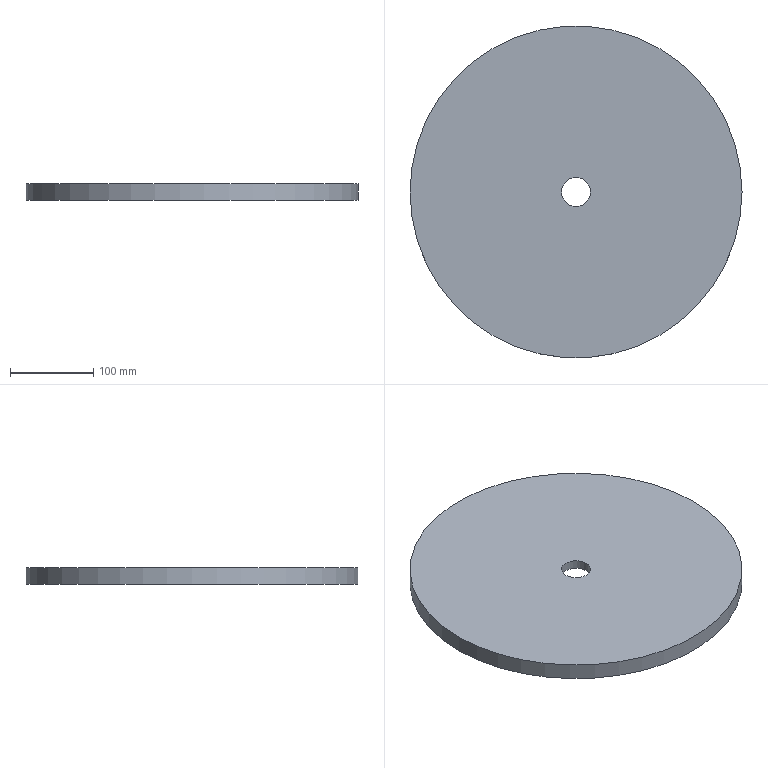Part | NX | features HOLE PACKAGE 6, SIMPLE HOLE 6, DATUM_CSYS 5, EXTRACT_DATUM_AXIS 4, EXTRACT_FACE 4, SKETCH 4, SYMBOLIC_THREAD 4, Instance Feature 3, CYLINDER 1, Pattern Feature 1 | 1 solid | 18 faces | box 400 x 400 x 20 mm | volume 2431329 mm3 | cone 8 | cylinder 7 | plane 3 | commonest cylinder face diameters 5 x4 35 x1 100 x1 400 x1
STEP:
#1=CARTESIAN_POINT('',(17.5,0.,20.));
#2=VERTEX_POINT('',#1);
#3=CARTESIAN_POINT('',(0.,0.,20.));
#4=DIRECTION('',(0.,0.,1.));
#5=DIRECTION('',(1.,0.,0.));
#6=AXIS2_PLACEMENT_3D('',#3,#4,#5);
#7=CIRCLE('',#6,17.5);
#8=EDGE_CURVE('',#2,#2,#7,.T.);
#9=ORIENTED_EDGE('',*,*,#8,.F.);
#10=EDGE_LOOP('',(#9));
#11=FACE_BOUND('',#10,.T.);
#12=CARTESIAN_POINT('',(200.,0.,20.));
#13=VERTEX_POINT('',#12);
#14=CARTESIAN_POINT('',(0.,0.,20.));
#15=DIRECTION('',(0.,0.,-1.));
#16=DIRECTION('',(1.,0.,0.));
#17=AXIS2_PLACEMENT_3D('',#14,#15,#16);
#18=CIRCLE('',#17,200.);
#19=EDGE_CURVE('',#13,#13,#18,.T.);
#20=ORIENTED_EDGE('',*,*,#19,.F.);
#21=EDGE_LOOP('',(#20));
#22=FACE_BOUND('',#21,.T.);
#23=CARTESIAN_POINT('',(0.,0.,20.));
#24=DIRECTION('',(0.,0.,1.));
#25=DIRECTION('',(1.,0.,0.));
#26=AXIS2_PLACEMENT_3D('',#23,#24,#25);
#27=PLANE('',#26);
#28=ADVANCED_FACE('',(#11,#22),#27,.T.);
#29=CARTESIAN_POINT('',(50.,0.,0.));
#30=VERTEX_POINT('',#29);
#31=CARTESIAN_POINT('',(0.,0.,0.));
#32=DIRECTION('',(0.,0.,1.));
#33=DIRECTION('',(1.,0.,0.));
#34=AXIS2_PLACEMENT_3D('',#31,#32,#33);
#35=CIRCLE('',#34,50.);
#36=EDGE_CURVE('',#30,#30,#35,.T.);
#37=ORIENTED_EDGE('',*,*,#36,.T.);
#38=EDGE_LOOP('',(#37));
#39=FACE_BOUND('',#38,.T.);
#40=CARTESIAN_POINT('',(200.,0.,0.));
#41=VERTEX_POINT('',#40);
#42=CARTESIAN_POINT('',(0.,0.,0.));
#43=DIRECTION('',(0.,0.,1.));
#44=DIRECTION('',(1.,0.,0.));
#45=AXIS2_PLACEMENT_3D('',#42,#43,#44);
#46=CIRCLE('',#45,200.);
#47=EDGE_CURVE('',#41,#41,#46,.T.);
#48=ORIENTED_EDGE('',*,*,#47,.F.);
#49=EDGE_LOOP('',(#48));
#50=FACE_BOUND('',#49,.T.);
#51=CARTESIAN_POINT('',(0.,0.,0.));
#52=DIRECTION('',(0.,0.,-1.));
#53=DIRECTION('',(-1.,0.,0.));
#54=AXIS2_PLACEMENT_3D('',#51,#52,#53);
#55=PLANE('',#54);
#56=ADVANCED_FACE('',(#39,#50),#55,.T.);
#57=ORIENTED_EDGE('',*,*,#19,.T.);
#58=EDGE_LOOP('',(#57));
#59=FACE_BOUND('',#58,.T.);
#60=ORIENTED_EDGE('',*,*,#47,.T.);
#61=EDGE_LOOP('',(#60));
#62=FACE_BOUND('',#61,.T.);
#63=CARTESIAN_POINT('',(0.,0.,0.));
#64=DIRECTION('',(0.,0.,1.));
#65=DIRECTION('',(1.,0.,0.));
#66=AXIS2_PLACEMENT_3D('',#63,#64,#65);
#67=CYLINDRICAL_SURFACE('',#66,200.);
#68=ADVANCED_FACE('',(#59,#62),#67,.T.);
#69=CARTESIAN_POINT('',(38.,0.,9.));
#70=VERTEX_POINT('',#69);
#71=CARTESIAN_POINT('',(35.,0.,9.));
#72=DIRECTION('',(0.,0.,1.));
#73=DIRECTION('',(1.,0.,0.));
#74=AXIS2_PLACEMENT_3D('',#71,#72,#73);
#75=CIRCLE('',#74,3.);
#76=EDGE_CURVE('',#70,#70,#75,.T.);
#77=ORIENTED_EDGE('',*,*,#76,.T.);
#78=EDGE_LOOP('',(#77));
#79=FACE_BOUND('',#78,.T.);
#80=CARTESIAN_POINT('',(3.,35.,9.));
#81=VERTEX_POINT('',#80);
#82=CARTESIAN_POINT('',(0.,35.,9.));
#83=DIRECTION('',(0.,0.,1.));
#84=DIRECTION('',(1.,0.,0.));
#85=AXIS2_PLACEMENT_3D('',#82,#83,#84);
#86=CIRCLE('',#85,3.);
#87=EDGE_CURVE('',#81,#81,#86,.T.);
#88=ORIENTED_EDGE('',*,*,#87,.T.);
#89=EDGE_LOOP('',(#88));
#90=FACE_BOUND('',#89,.T.);
#91=CARTESIAN_POINT('',(-32.,0.,9.));
#92=VERTEX_POINT('',#91);
#93=CARTESIAN_POINT('',(-35.,0.,9.));
#94=DIRECTION('',(0.,0.,1.));
#95=DIRECTION('',(1.,0.,0.));
#96=AXIS2_PLACEMENT_3D('',#93,#94,#95);
#97=CIRCLE('',#96,3.);
#98=EDGE_CURVE('',#92,#92,#97,.T.);
#99=ORIENTED_EDGE('',*,*,#98,.T.);
#100=EDGE_LOOP('',(#99));
#101=FACE_BOUND('',#100,.T.);
#102=CARTESIAN_POINT('',(3.,-35.,9.));
#103=VERTEX_POINT('',#102);
#104=CARTESIAN_POINT('',(0.,-35.,9.));
#105=DIRECTION('',(0.,0.,1.));
#106=DIRECTION('',(1.,0.,0.));
#107=AXIS2_PLACEMENT_3D('',#104,#105,#106);
#108=CIRCLE('',#107,3.);
#109=EDGE_CURVE('',#103,#103,#108,.T.);
#110=ORIENTED_EDGE('',*,*,#109,.T.);
#111=EDGE_LOOP('',(#110));
#112=FACE_BOUND('',#111,.T.);
#113=CARTESIAN_POINT('',(17.5,0.,9.));
#114=VERTEX_POINT('',#113);
#115=CARTESIAN_POINT('',(0.,0.,9.));
#116=DIRECTION('',(0.,0.,1.));
#117=DIRECTION('',(1.,0.,0.));
#118=AXIS2_PLACEMENT_3D('',#115,#116,#117);
#119=CIRCLE('',#118,17.5);
#120=EDGE_CURVE('',#114,#114,#119,.T.);
#121=ORIENTED_EDGE('',*,*,#120,.T.);
#122=EDGE_LOOP('',(#121));
#123=FACE_BOUND('',#122,.T.);
#124=CARTESIAN_POINT('',(50.,0.,9.));
#125=VERTEX_POINT('',#124);
#126=CARTESIAN_POINT('',(0.,0.,9.));
#127=DIRECTION('',(0.,0.,1.));
#128=DIRECTION('',(1.,0.,0.));
#129=AXIS2_PLACEMENT_3D('',#126,#127,#128);
#130=CIRCLE('',#129,50.);
#131=EDGE_CURVE('',#125,#125,#130,.F.);
#132=ORIENTED_EDGE('',*,*,#131,.T.);
#133=EDGE_LOOP('',(#132));
#134=FACE_BOUND('',#133,.T.);
#135=CARTESIAN_POINT('',(0.,0.,9.));
#136=DIRECTION('',(0.,0.,1.));
#137=DIRECTION('',(1.,0.,0.));
#138=AXIS2_PLACEMENT_3D('',#135,#136,#137);
#139=PLANE('',#138);
#140=ADVANCED_FACE('',(#79,#90,#101,#112,#123,#134),#139,.F.);
#141=ORIENTED_EDGE('',*,*,#131,.F.);
#142=EDGE_LOOP('',(#141));
#143=FACE_BOUND('',#142,.T.);
#144=ORIENTED_EDGE('',*,*,#36,.F.);
#145=EDGE_LOOP('',(#144));
#146=FACE_BOUND('',#145,.T.);
#147=CARTESIAN_POINT('',(0.,0.,0.));
#148=DIRECTION('',(0.,0.,1.));
#149=DIRECTION('',(1.,0.,0.));
#150=AXIS2_PLACEMENT_3D('',#147,#148,#149);
#151=CYLINDRICAL_SURFACE('',#150,50.);
#152=ADVANCED_FACE('',(#143,#146),#151,.F.);
#153=ORIENTED_EDGE('',*,*,#8,.T.);
#154=EDGE_LOOP('',(#153));
#155=FACE_BOUND('',#154,.T.);
#156=ORIENTED_EDGE('',*,*,#120,.F.);
#157=EDGE_LOOP('',(#156));
#158=FACE_BOUND('',#157,.T.);
#159=CARTESIAN_POINT('',(0.,0.,9.));
#160=DIRECTION('',(0.,0.,1.));
#161=DIRECTION('',(1.,0.,0.));
#162=AXIS2_PLACEMENT_3D('',#159,#160,#161);
#163=CYLINDRICAL_SURFACE('',#162,17.5);
#164=ADVANCED_FACE('',(#155,#158),#163,.F.);
#165=CARTESIAN_POINT('',(2.5,-35.,17.));
#166=VERTEX_POINT('',#165);
#167=CARTESIAN_POINT('',(0.,-35.,17.));
#168=DIRECTION('',(0.,0.,1.));
#169=DIRECTION('',(1.,0.,0.));
#170=AXIS2_PLACEMENT_3D('',#167,#168,#169);
#171=CIRCLE('',#170,2.5);
#172=EDGE_CURVE('',#166,#166,#171,.F.);
#173=ORIENTED_EDGE('',*,*,#172,.T.);
#174=EDGE_LOOP('',(#173));
#175=FACE_BOUND('',#174,.T.);
#176=CARTESIAN_POINT('',(0.,-35.,18.502));
#177=VERTEX_POINT('',#176);
#178=VERTEX_LOOP('',#177);
#179=FACE_BOUND('',#178,.T.);
#180=CARTESIAN_POINT('',(0.,-35.,17.));
#181=DIRECTION('',(0.,0.,-1.));
#182=DIRECTION('',(-1.,0.,0.));
#183=AXIS2_PLACEMENT_3D('',#180,#181,#182);
#184=CONICAL_SURFACE('',#183,2.5,1.03);
#185=ADVANCED_FACE('',(#175,#179),#184,.F.);
#186=CARTESIAN_POINT('',(2.5,-35.,9.5));
#187=VERTEX_POINT('',#186);
#188=CARTESIAN_POINT('',(0.,-35.,9.5));
#189=DIRECTION('',(0.,0.,1.));
#190=DIRECTION('',(1.,0.,0.));
#191=AXIS2_PLACEMENT_3D('',#188,#189,#190);
#192=CIRCLE('',#191,2.5);
#193=EDGE_CURVE('',#187,#187,#192,.F.);
#194=ORIENTED_EDGE('',*,*,#193,.T.);
#195=EDGE_LOOP('',(#194));
#196=FACE_BOUND('',#195,.T.);
#197=ORIENTED_EDGE('',*,*,#172,.F.);
#198=EDGE_LOOP('',(#197));
#199=FACE_BOUND('',#198,.T.);
#200=CARTESIAN_POINT('',(0.,-35.,9.));
#201=DIRECTION('',(0.,0.,1.));
#202=DIRECTION('',(1.,0.,0.));
#203=AXIS2_PLACEMENT_3D('',#200,#201,#202);
#204=CYLINDRICAL_SURFACE('',#203,2.5);
#205=ADVANCED_FACE('',(#196,#199),#204,.F.);
#206=ORIENTED_EDGE('',*,*,#193,.F.);
#207=EDGE_LOOP('',(#206));
#208=FACE_BOUND('',#207,.T.);
#209=ORIENTED_EDGE('',*,*,#109,.F.);
#210=EDGE_LOOP('',(#209));
#211=FACE_BOUND('',#210,.T.);
#212=CARTESIAN_POINT('',(0.,-35.,9.));
#213=DIRECTION('',(0.,0.,-1.));
#214=DIRECTION('',(-1.,0.,0.));
#215=AXIS2_PLACEMENT_3D('',#212,#213,#214);
#216=CONICAL_SURFACE('',#215,3.,0.7854);
#217=ADVANCED_FACE('',(#208,#211),#216,.F.);
#218=CARTESIAN_POINT('',(-32.5,0.,17.));
#219=VERTEX_POINT('',#218);
#220=CARTESIAN_POINT('',(-35.,0.,17.));
#221=DIRECTION('',(0.,0.,1.));
#222=DIRECTION('',(1.,0.,0.));
#223=AXIS2_PLACEMENT_3D('',#220,#221,#222);
#224=CIRCLE('',#223,2.5);
#225=EDGE_CURVE('',#219,#219,#224,.F.);
#226=ORIENTED_EDGE('',*,*,#225,.T.);
#227=EDGE_LOOP('',(#226));
#228=FACE_BOUND('',#227,.T.);
#229=CARTESIAN_POINT('',(-35.,0.,18.502));
#230=VERTEX_POINT('',#229);
#231=VERTEX_LOOP('',#230);
#232=FACE_BOUND('',#231,.T.);
#233=CARTESIAN_POINT('',(-35.,0.,17.));
#234=DIRECTION('',(0.,0.,-1.));
#235=DIRECTION('',(-1.,0.,0.));
#236=AXIS2_PLACEMENT_3D('',#233,#234,#235);
#237=CONICAL_SURFACE('',#236,2.5,1.03);
#238=ADVANCED_FACE('',(#228,#232),#237,.F.);
#239=CARTESIAN_POINT('',(-32.5,0.,9.5));
#240=VERTEX_POINT('',#239);
#241=CARTESIAN_POINT('',(-35.,0.,9.5));
#242=DIRECTION('',(0.,0.,1.));
#243=DIRECTION('',(1.,0.,0.));
#244=AXIS2_PLACEMENT_3D('',#241,#242,#243);
#245=CIRCLE('',#244,2.5);
#246=EDGE_CURVE('',#240,#240,#245,.F.);
#247=ORIENTED_EDGE('',*,*,#246,.T.);
#248=EDGE_LOOP('',(#247));
#249=FACE_BOUND('',#248,.T.);
#250=ORIENTED_EDGE('',*,*,#225,.F.);
#251=EDGE_LOOP('',(#250));
#252=FACE_BOUND('',#251,.T.);
#253=CARTESIAN_POINT('',(-35.,0.,9.));
#254=DIRECTION('',(0.,0.,1.));
#255=DIRECTION('',(1.,0.,0.));
#256=AXIS2_PLACEMENT_3D('',#253,#254,#255);
#257=CYLINDRICAL_SURFACE('',#256,2.5);
#258=ADVANCED_FACE('',(#249,#252),#257,.F.);
#259=ORIENTED_EDGE('',*,*,#246,.F.);
#260=EDGE_LOOP('',(#259));
#261=FACE_BOUND('',#260,.T.);
#262=ORIENTED_EDGE('',*,*,#98,.F.);
#263=EDGE_LOOP('',(#262));
#264=FACE_BOUND('',#263,.T.);
#265=CARTESIAN_POINT('',(-35.,0.,9.));
#266=DIRECTION('',(0.,0.,-1.));
#267=DIRECTION('',(-1.,0.,0.));
#268=AXIS2_PLACEMENT_3D('',#265,#266,#267);
#269=CONICAL_SURFACE('',#268,3.,0.7854);
#270=ADVANCED_FACE('',(#261,#264),#269,.F.);
#271=CARTESIAN_POINT('',(2.5,35.,17.));
#272=VERTEX_POINT('',#271);
#273=CARTESIAN_POINT('',(0.,35.,17.));
#274=DIRECTION('',(0.,0.,1.));
#275=DIRECTION('',(1.,0.,0.));
#276=AXIS2_PLACEMENT_3D('',#273,#274,#275);
#277=CIRCLE('',#276,2.5);
#278=EDGE_CURVE('',#272,#272,#277,.F.);
#279=ORIENTED_EDGE('',*,*,#278,.T.);
#280=EDGE_LOOP('',(#279));
#281=FACE_BOUND('',#280,.T.);
#282=CARTESIAN_POINT('',(0.,35.,18.502));
#283=VERTEX_POINT('',#282);
#284=VERTEX_LOOP('',#283);
#285=FACE_BOUND('',#284,.T.);
#286=CARTESIAN_POINT('',(0.,35.,17.));
#287=DIRECTION('',(0.,0.,-1.));
#288=DIRECTION('',(-1.,0.,0.));
#289=AXIS2_PLACEMENT_3D('',#286,#287,#288);
#290=CONICAL_SURFACE('',#289,2.5,1.03);
#291=ADVANCED_FACE('',(#281,#285),#290,.F.);
#292=CARTESIAN_POINT('',(2.5,35.,9.5));
#293=VERTEX_POINT('',#292);
#294=CARTESIAN_POINT('',(0.,35.,9.5));
#295=DIRECTION('',(0.,0.,1.));
#296=DIRECTION('',(1.,0.,0.));
#297=AXIS2_PLACEMENT_3D('',#294,#295,#296);
#298=CIRCLE('',#297,2.5);
#299=EDGE_CURVE('',#293,#293,#298,.F.);
#300=ORIENTED_EDGE('',*,*,#299,.T.);
#301=EDGE_LOOP('',(#300));
#302=FACE_BOUND('',#301,.T.);
#303=ORIENTED_EDGE('',*,*,#278,.F.);
#304=EDGE_LOOP('',(#303));
#305=FACE_BOUND('',#304,.T.);
#306=CARTESIAN_POINT('',(0.,35.,9.));
#307=DIRECTION('',(0.,0.,1.));
#308=DIRECTION('',(1.,0.,0.));
#309=AXIS2_PLACEMENT_3D('',#306,#307,#308);
#310=CYLINDRICAL_SURFACE('',#309,2.5);
#311=ADVANCED_FACE('',(#302,#305),#310,.F.);
#312=ORIENTED_EDGE('',*,*,#299,.F.);
#313=EDGE_LOOP('',(#312));
#314=FACE_BOUND('',#313,.T.);
#315=ORIENTED_EDGE('',*,*,#87,.F.);
#316=EDGE_LOOP('',(#315));
#317=FACE_BOUND('',#316,.T.);
#318=CARTESIAN_POINT('',(0.,35.,9.));
#319=DIRECTION('',(0.,0.,-1.));
#320=DIRECTION('',(-1.,0.,0.));
#321=AXIS2_PLACEMENT_3D('',#318,#319,#320);
#322=CONICAL_SURFACE('',#321,3.,0.7854);
#323=ADVANCED_FACE('',(#314,#317),#322,.F.);
#324=CARTESIAN_POINT('',(37.5,0.,17.));
#325=VERTEX_POINT('',#324);
#326=CARTESIAN_POINT('',(35.,0.,17.));
#327=DIRECTION('',(0.,0.,1.));
#328=DIRECTION('',(1.,0.,0.));
#329=AXIS2_PLACEMENT_3D('',#326,#327,#328);
#330=CIRCLE('',#329,2.5);
#331=EDGE_CURVE('',#325,#325,#330,.F.);
#332=ORIENTED_EDGE('',*,*,#331,.T.);
#333=EDGE_LOOP('',(#332));
#334=FACE_BOUND('',#333,.T.);
#335=CARTESIAN_POINT('',(35.,0.,18.502));
#336=VERTEX_POINT('',#335);
#337=VERTEX_LOOP('',#336);
#338=FACE_BOUND('',#337,.T.);
#339=CARTESIAN_POINT('',(35.,0.,17.));
#340=DIRECTION('',(0.,0.,-1.));
#341=DIRECTION('',(-1.,0.,0.));
#342=AXIS2_PLACEMENT_3D('',#339,#340,#341);
#343=CONICAL_SURFACE('',#342,2.5,1.03);
#344=ADVANCED_FACE('',(#334,#338),#343,.F.);
#345=CARTESIAN_POINT('',(37.5,0.,9.5));
#346=VERTEX_POINT('',#345);
#347=CARTESIAN_POINT('',(35.,0.,9.5));
#348=DIRECTION('',(0.,0.,1.));
#349=DIRECTION('',(1.,0.,0.));
#350=AXIS2_PLACEMENT_3D('',#347,#348,#349);
#351=CIRCLE('',#350,2.5);
#352=EDGE_CURVE('',#346,#346,#351,.F.);
#353=ORIENTED_EDGE('',*,*,#352,.T.);
#354=EDGE_LOOP('',(#353));
#355=FACE_BOUND('',#354,.T.);
#356=ORIENTED_EDGE('',*,*,#331,.F.);
#357=EDGE_LOOP('',(#356));
#358=FACE_BOUND('',#357,.T.);
#359=CARTESIAN_POINT('',(35.,0.,9.));
#360=DIRECTION('',(0.,0.,1.));
#361=DIRECTION('',(1.,0.,0.));
#362=AXIS2_PLACEMENT_3D('',#359,#360,#361);
#363=CYLINDRICAL_SURFACE('',#362,2.5);
#364=ADVANCED_FACE('',(#355,#358),#363,.F.);
#365=ORIENTED_EDGE('',*,*,#352,.F.);
#366=EDGE_LOOP('',(#365));
#367=FACE_BOUND('',#366,.T.);
#368=ORIENTED_EDGE('',*,*,#76,.F.);
#369=EDGE_LOOP('',(#368));
#370=FACE_BOUND('',#369,.T.);
#371=CARTESIAN_POINT('',(35.,0.,9.));
#372=DIRECTION('',(0.,0.,-1.));
#373=DIRECTION('',(-1.,0.,0.));
#374=AXIS2_PLACEMENT_3D('',#371,#372,#373);
#375=CONICAL_SURFACE('',#374,3.,0.7854);
#376=ADVANCED_FACE('',(#367,#370),#375,.F.);
#377=CLOSED_SHELL('',(#28,#56,#68,#140,#152,#164,#185,#205,#217,#238,#258,#270,#291,#311,#323,#344,#364,#376));
#378=MANIFOLD_SOLID_BREP('',#377);
#379=(LENGTH_UNIT()NAMED_UNIT(*)SI_UNIT(.MILLI.,.METRE.));
#380=UNCERTAINTY_MEASURE_WITH_UNIT(LENGTH_MEASURE(0.00001),#379,'','');
#381=(NAMED_UNIT(*)PLANE_ANGLE_UNIT()SI_UNIT($,.RADIAN.));
#382=(NAMED_UNIT(*)SI_UNIT($,.STERADIAN.)SOLID_ANGLE_UNIT());
#383=(GEOMETRIC_REPRESENTATION_CONTEXT(3)GLOBAL_UNCERTAINTY_ASSIGNED_CONTEXT((#380))GLOBAL_UNIT_ASSIGNED_CONTEXT((#379,#381,#382))REPRESENTATION_CONTEXT('',''));
#384=ADVANCED_BREP_SHAPE_REPRESENTATION('',(#378),#383);